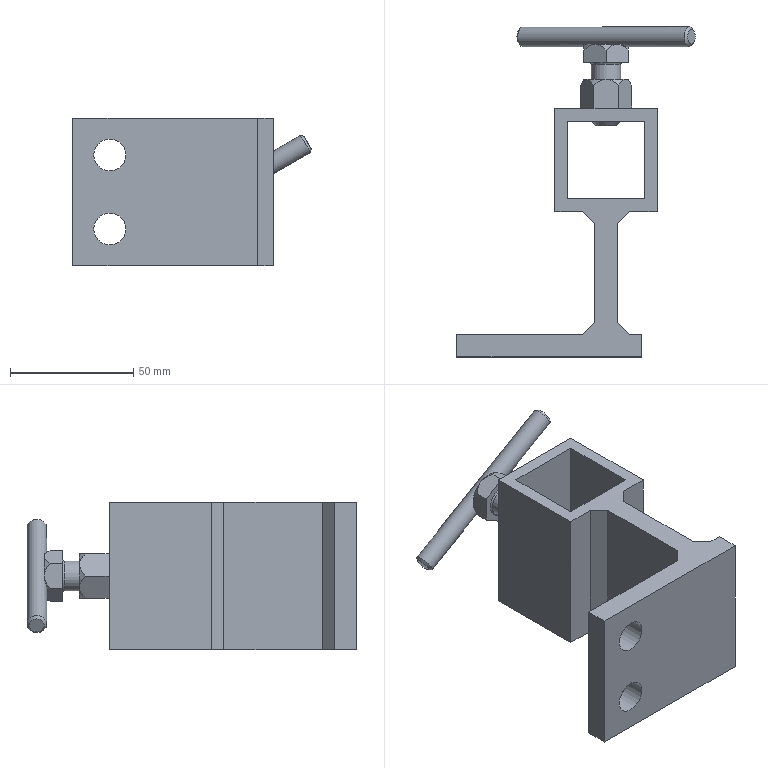Part | NX | features solid 2 | 1 solid | 66 faces | box 96.641 x 133.8 x 60 mm | volume 122041 mm3 | plane 42 | cone 17 | cylinder 6 | torus 1 | commonest cylinder face diameters 13 x3 12 x2 8 x1